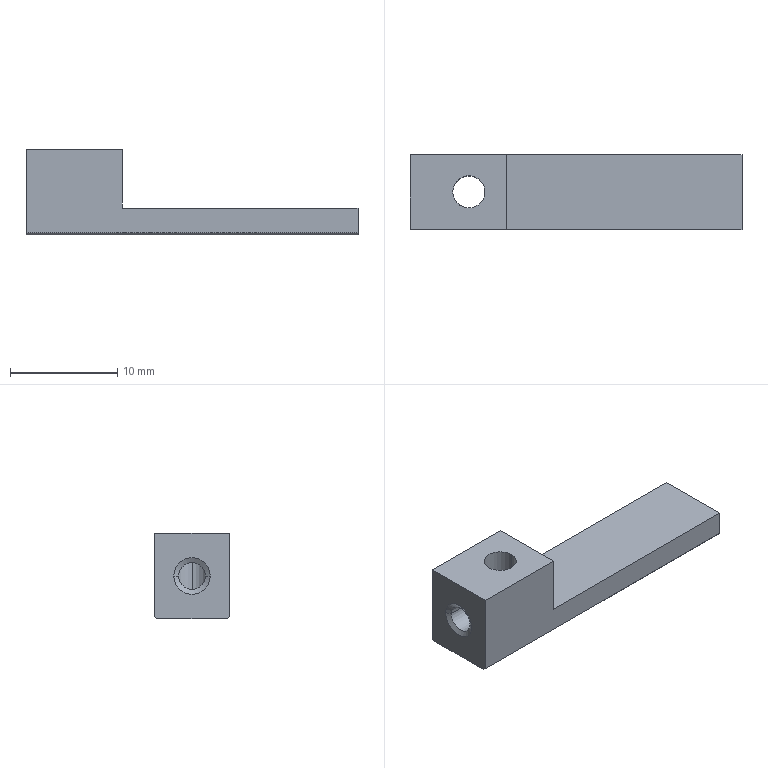Part | NX | 1 solid | 16 faces | box 31 x 7 x 8 mm | volume 810.336 mm3 | plane 10 | cylinder 4 | cone 2 | commonest cylinder face diameters 2.5 x2 3 x2
STEP:
#1=CARTESIAN_POINT('',(15.5,-3.3,-4.));
#2=VERTEX_POINT('',#1);
#3=CARTESIAN_POINT('',(-15.5,-3.3,-4.));
#4=VERTEX_POINT('',#3);
#5=CARTESIAN_POINT('',(0.,-3.3,-4.));
#6=DIRECTION('',(-1.,0.,0.));
#7=VECTOR('',#6,1000.);
#8=LINE('',#5,#7);
#9=EDGE_CURVE('',#2,#4,#8,.T.);
#10=ORIENTED_EDGE('',*,*,#9,.T.);
#11=CARTESIAN_POINT('',(-15.5,3.3,-4.));
#12=VERTEX_POINT('',#11);
#13=CARTESIAN_POINT('',(-15.5,0.,-4.));
#14=DIRECTION('',(0.,-1.,0.));
#15=VECTOR('',#14,1000.);
#16=LINE('',#13,#15);
#17=EDGE_CURVE('',#12,#4,#16,.T.);
#18=ORIENTED_EDGE('',*,*,#17,.F.);
#19=CARTESIAN_POINT('',(15.5,3.3,-4.));
#20=VERTEX_POINT('',#19);
#21=CARTESIAN_POINT('',(0.,3.3,-4.));
#22=DIRECTION('',(1.,0.,0.));
#23=VECTOR('',#22,1000.);
#24=LINE('',#21,#23);
#25=EDGE_CURVE('',#12,#20,#24,.T.);
#26=ORIENTED_EDGE('',*,*,#25,.T.);
#27=CARTESIAN_POINT('',(15.5,3.5,-4.));
#28=DIRECTION('',(0.,-1.,0.));
#29=VECTOR('',#28,1000.);
#30=LINE('',#27,#29);
#31=EDGE_CURVE('',#20,#2,#30,.T.);
#32=ORIENTED_EDGE('',*,*,#31,.T.);
#33=EDGE_LOOP('',(#10,#18,#26,#32));
#34=FACE_BOUND('',#33,.T.);
#35=CARTESIAN_POINT('',(-11.5,0.,-4.));
#36=VERTEX_POINT('',#35);
#37=CARTESIAN_POINT('',(-8.5,0.,-4.));
#38=VERTEX_POINT('',#37);
#39=CARTESIAN_POINT('',(-10.,0.,-4.));
#40=DIRECTION('',(0.,0.,1.));
#41=DIRECTION('',(1.,0.,0.));
#42=AXIS2_PLACEMENT_3D('',#39,#40,#41);
#43=CIRCLE('',#42,1.5);
#44=EDGE_CURVE('',#36,#38,#43,.T.);
#45=ORIENTED_EDGE('',*,*,#44,.T.);
#46=CARTESIAN_POINT('',(-10.,0.,-4.));
#47=DIRECTION('',(0.,0.,1.));
#48=DIRECTION('',(1.,0.,0.));
#49=AXIS2_PLACEMENT_3D('',#46,#47,#48);
#50=CIRCLE('',#49,1.5);
#51=EDGE_CURVE('',#38,#36,#50,.T.);
#52=ORIENTED_EDGE('',*,*,#51,.T.);
#53=EDGE_LOOP('',(#45,#52));
#54=FACE_BOUND('',#53,.T.);
#55=CARTESIAN_POINT('',(0.,0.,-4.));
#56=DIRECTION('',(0.,0.,1.));
#57=DIRECTION('',(1.,0.,0.));
#58=AXIS2_PLACEMENT_3D('',#55,#56,#57);
#59=PLANE('',#58);
#60=ADVANCED_FACE('',(#34,#54),#59,.F.);
#61=ORIENTED_EDGE('',*,*,#17,.T.);
#62=CARTESIAN_POINT('',(-15.5,-3.5,-3.8));
#63=VERTEX_POINT('',#62);
#64=CARTESIAN_POINT('',(-15.5,-7.3,0.));
#65=DIRECTION('',(0.,0.7071,-0.7071));
#66=VECTOR('',#65,1000.);
#67=LINE('',#64,#66);
#68=EDGE_CURVE('',#63,#4,#67,.T.);
#69=ORIENTED_EDGE('',*,*,#68,.F.);
#70=CARTESIAN_POINT('',(-15.5,-3.5,4.));
#71=VERTEX_POINT('',#70);
#72=CARTESIAN_POINT('',(-15.5,-3.5,0.));
#73=DIRECTION('',(0.,0.,-1.));
#74=VECTOR('',#73,1000.);
#75=LINE('',#72,#74);
#76=EDGE_CURVE('',#71,#63,#75,.T.);
#77=ORIENTED_EDGE('',*,*,#76,.F.);
#78=CARTESIAN_POINT('',(-15.5,3.5,4.));
#79=VERTEX_POINT('',#78);
#80=CARTESIAN_POINT('',(-15.5,0.,4.));
#81=DIRECTION('',(0.,-1.,0.));
#82=VECTOR('',#81,1000.);
#83=LINE('',#80,#82);
#84=EDGE_CURVE('',#79,#71,#83,.T.);
#85=ORIENTED_EDGE('',*,*,#84,.F.);
#86=CARTESIAN_POINT('',(-15.5,3.5,-3.8));
#87=VERTEX_POINT('',#86);
#88=CARTESIAN_POINT('',(-15.5,3.5,0.));
#89=DIRECTION('',(0.,0.,1.));
#90=VECTOR('',#89,1000.);
#91=LINE('',#88,#90);
#92=EDGE_CURVE('',#87,#79,#91,.T.);
#93=ORIENTED_EDGE('',*,*,#92,.F.);
#94=CARTESIAN_POINT('',(-15.5,7.3,0.));
#95=DIRECTION('',(0.,0.7071,0.7071));
#96=VECTOR('',#95,1000.);
#97=LINE('',#94,#96);
#98=EDGE_CURVE('',#12,#87,#97,.T.);
#99=ORIENTED_EDGE('',*,*,#98,.F.);
#100=EDGE_LOOP('',(#61,#69,#77,#85,#93,#99));
#101=FACE_BOUND('',#100,.T.);
#102=CARTESIAN_POINT('',(-15.5,1.7,0.));
#103=VERTEX_POINT('',#102);
#104=CARTESIAN_POINT('',(-15.5,-1.7,0.));
#105=VERTEX_POINT('',#104);
#106=CARTESIAN_POINT('',(-15.5,0.,0.));
#107=DIRECTION('',(-1.,0.,0.));
#108=DIRECTION('',(0.,1.,0.));
#109=AXIS2_PLACEMENT_3D('',#106,#107,#108);
#110=CIRCLE('',#109,1.7);
#111=EDGE_CURVE('',#103,#105,#110,.T.);
#112=ORIENTED_EDGE('',*,*,#111,.F.);
#113=CARTESIAN_POINT('',(-15.5,0.,0.));
#114=DIRECTION('',(-1.,0.,0.));
#115=DIRECTION('',(0.,1.,0.));
#116=AXIS2_PLACEMENT_3D('',#113,#114,#115);
#117=CIRCLE('',#116,1.7);
#118=EDGE_CURVE('',#105,#103,#117,.T.);
#119=ORIENTED_EDGE('',*,*,#118,.F.);
#120=EDGE_LOOP('',(#112,#119));
#121=FACE_BOUND('',#120,.T.);
#122=CARTESIAN_POINT('',(-15.5,3.5,-4.));
#123=DIRECTION('',(-1.,0.,0.));
#124=DIRECTION('',(0.,0.,1.));
#125=AXIS2_PLACEMENT_3D('',#122,#123,#124);
#126=PLANE('',#125);
#127=ADVANCED_FACE('',(#101,#121),#126,.T.);
#128=CARTESIAN_POINT('',(-6.5,3.5,-1.5));
#129=VERTEX_POINT('',#128);
#130=CARTESIAN_POINT('',(15.5,3.5,-1.5));
#131=VERTEX_POINT('',#130);
#132=CARTESIAN_POINT('',(-6.5,3.5,-1.5));
#133=DIRECTION('',(1.,0.,0.));
#134=VECTOR('',#133,1000.);
#135=LINE('',#132,#134);
#136=EDGE_CURVE('',#129,#131,#135,.T.);
#137=ORIENTED_EDGE('',*,*,#136,.T.);
#138=CARTESIAN_POINT('',(15.5,3.5,-3.8));
#139=VERTEX_POINT('',#138);
#140=CARTESIAN_POINT('',(15.5,3.5,-1.5));
#141=DIRECTION('',(0.,0.,-1.));
#142=VECTOR('',#141,1000.);
#143=LINE('',#140,#142);
#144=EDGE_CURVE('',#131,#139,#143,.T.);
#145=ORIENTED_EDGE('',*,*,#144,.T.);
#146=CARTESIAN_POINT('',(0.,3.5,-3.8));
#147=DIRECTION('',(1.,0.,0.));
#148=VECTOR('',#147,1000.);
#149=LINE('',#146,#148);
#150=EDGE_CURVE('',#87,#139,#149,.T.);
#151=ORIENTED_EDGE('',*,*,#150,.F.);
#152=ORIENTED_EDGE('',*,*,#92,.T.);
#153=CARTESIAN_POINT('',(-6.5,3.5,4.));
#154=VERTEX_POINT('',#153);
#155=CARTESIAN_POINT('',(-15.5,3.5,4.));
#156=DIRECTION('',(1.,0.,0.));
#157=VECTOR('',#156,1000.);
#158=LINE('',#155,#157);
#159=EDGE_CURVE('',#79,#154,#158,.T.);
#160=ORIENTED_EDGE('',*,*,#159,.T.);
#161=CARTESIAN_POINT('',(-6.5,3.5,-1.5));
#162=DIRECTION('',(0.,0.,1.));
#163=VECTOR('',#162,1000.);
#164=LINE('',#161,#163);
#165=EDGE_CURVE('',#129,#154,#164,.T.);
#166=ORIENTED_EDGE('',*,*,#165,.F.);
#167=EDGE_LOOP('',(#137,#145,#151,#152,#160,#166));
#168=FACE_BOUND('',#167,.T.);
#169=CARTESIAN_POINT('',(15.5,3.5,-4.));
#170=DIRECTION('',(0.,1.,0.));
#171=DIRECTION('',(1.,0.,0.));
#172=AXIS2_PLACEMENT_3D('',#169,#170,#171);
#173=PLANE('',#172);
#174=ADVANCED_FACE('',(#168),#173,.T.);
#175=CARTESIAN_POINT('',(-6.5,-3.5,-1.5));
#176=VERTEX_POINT('',#175);
#177=CARTESIAN_POINT('',(15.5,-3.5,-1.5));
#178=VERTEX_POINT('',#177);
#179=CARTESIAN_POINT('',(-6.5,-3.5,-1.5));
#180=DIRECTION('',(1.,0.,0.));
#181=VECTOR('',#180,1000.);
#182=LINE('',#179,#181);
#183=EDGE_CURVE('',#176,#178,#182,.T.);
#184=ORIENTED_EDGE('',*,*,#183,.T.);
#185=CARTESIAN_POINT('',(15.5,3.5,-1.5));
#186=DIRECTION('',(0.,-1.,0.));
#187=VECTOR('',#186,1000.);
#188=LINE('',#185,#187);
#189=EDGE_CURVE('',#131,#178,#188,.T.);
#190=ORIENTED_EDGE('',*,*,#189,.F.);
#191=ORIENTED_EDGE('',*,*,#136,.F.);
#192=CARTESIAN_POINT('',(-6.5,-3.5,-1.5));
#193=DIRECTION('',(0.,1.,0.));
#194=VECTOR('',#193,1000.);
#195=LINE('',#192,#194);
#196=EDGE_CURVE('',#176,#129,#195,.T.);
#197=ORIENTED_EDGE('',*,*,#196,.F.);
#198=EDGE_LOOP('',(#184,#190,#191,#197));
#199=FACE_BOUND('',#198,.T.);
#200=CARTESIAN_POINT('',(15.5,3.5,-1.5));
#201=DIRECTION('',(0.,0.,-1.));
#202=DIRECTION('',(0.,-1.,0.));
#203=AXIS2_PLACEMENT_3D('',#200,#201,#202);
#204=PLANE('',#203);
#205=ADVANCED_FACE('',(#199),#204,.F.);
#206=ORIENTED_EDGE('',*,*,#183,.F.);
#207=CARTESIAN_POINT('',(-6.5,-3.5,4.));
#208=VERTEX_POINT('',#207);
#209=CARTESIAN_POINT('',(-6.5,-3.5,-1.5));
#210=DIRECTION('',(0.,0.,1.));
#211=VECTOR('',#210,1000.);
#212=LINE('',#209,#211);
#213=EDGE_CURVE('',#176,#208,#212,.T.);
#214=ORIENTED_EDGE('',*,*,#213,.T.);
#215=CARTESIAN_POINT('',(-6.5,-3.5,4.));
#216=DIRECTION('',(-1.,0.,0.));
#217=VECTOR('',#216,1000.);
#218=LINE('',#215,#217);
#219=EDGE_CURVE('',#208,#71,#218,.T.);
#220=ORIENTED_EDGE('',*,*,#219,.T.);
#221=ORIENTED_EDGE('',*,*,#76,.T.);
#222=CARTESIAN_POINT('',(15.5,-3.5,-3.8));
#223=VERTEX_POINT('',#222);
#224=CARTESIAN_POINT('',(0.,-3.5,-3.8));
#225=DIRECTION('',(-1.,0.,0.));
#226=VECTOR('',#225,1000.);
#227=LINE('',#224,#226);
#228=EDGE_CURVE('',#223,#63,#227,.T.);
#229=ORIENTED_EDGE('',*,*,#228,.F.);
#230=CARTESIAN_POINT('',(15.5,-3.5,-1.5));
#231=DIRECTION('',(0.,0.,-1.));
#232=VECTOR('',#231,1000.);
#233=LINE('',#230,#232);
#234=EDGE_CURVE('',#178,#223,#233,.T.);
#235=ORIENTED_EDGE('',*,*,#234,.F.);
#236=EDGE_LOOP('',(#206,#214,#220,#221,#229,#235));
#237=FACE_BOUND('',#236,.T.);
#238=CARTESIAN_POINT('',(-15.5,-3.5,-4.));
#239=DIRECTION('',(0.,-1.,0.));
#240=DIRECTION('',(0.,0.,-1.));
#241=AXIS2_PLACEMENT_3D('',#238,#239,#240);
#242=PLANE('',#241);
#243=ADVANCED_FACE('',(#237),#242,.T.);
#244=ORIENTED_EDGE('',*,*,#189,.T.);
#245=ORIENTED_EDGE('',*,*,#234,.T.);
#246=CARTESIAN_POINT('',(15.5,-7.3,0.));
#247=DIRECTION('',(0.,-0.7071,0.7071));
#248=VECTOR('',#247,1000.);
#249=LINE('',#246,#248);
#250=EDGE_CURVE('',#2,#223,#249,.T.);
#251=ORIENTED_EDGE('',*,*,#250,.F.);
#252=ORIENTED_EDGE('',*,*,#31,.F.);
#253=CARTESIAN_POINT('',(15.5,7.3,0.));
#254=DIRECTION('',(0.,-0.7071,-0.7071));
#255=VECTOR('',#254,1000.);
#256=LINE('',#253,#255);
#257=EDGE_CURVE('',#139,#20,#256,.T.);
#258=ORIENTED_EDGE('',*,*,#257,.F.);
#259=ORIENTED_EDGE('',*,*,#144,.F.);
#260=EDGE_LOOP('',(#244,#245,#251,#252,#258,#259));
#261=FACE_BOUND('',#260,.T.);
#262=CARTESIAN_POINT('',(15.5,-3.5,-4.));
#263=DIRECTION('',(1.,0.,0.));
#264=DIRECTION('',(0.,1.,0.));
#265=AXIS2_PLACEMENT_3D('',#262,#263,#264);
#266=PLANE('',#265);
#267=ADVANCED_FACE('',(#261),#266,.T.);
#268=CARTESIAN_POINT('',(-6.5,3.5,4.));
#269=DIRECTION('',(0.,-1.,0.));
#270=VECTOR('',#269,1000.);
#271=LINE('',#268,#270);
#272=EDGE_CURVE('',#154,#208,#271,.T.);
#273=ORIENTED_EDGE('',*,*,#272,.F.);
#274=ORIENTED_EDGE('',*,*,#159,.F.);
#275=ORIENTED_EDGE('',*,*,#84,.T.);
#276=ORIENTED_EDGE('',*,*,#219,.F.);
#277=EDGE_LOOP('',(#273,#274,#275,#276));
#278=FACE_BOUND('',#277,.T.);
#279=CARTESIAN_POINT('',(-8.5,0.,4.));
#280=VERTEX_POINT('',#279);
#281=CARTESIAN_POINT('',(-11.5,0.,4.));
#282=VERTEX_POINT('',#281);
#283=CARTESIAN_POINT('',(-10.,0.,4.));
#284=DIRECTION('',(0.,0.,1.));
#285=DIRECTION('',(1.,0.,0.));
#286=AXIS2_PLACEMENT_3D('',#283,#284,#285);
#287=CIRCLE('',#286,1.5);
#288=EDGE_CURVE('',#280,#282,#287,.T.);
#289=ORIENTED_EDGE('',*,*,#288,.F.);
#290=CARTESIAN_POINT('',(-10.,0.,4.));
#291=DIRECTION('',(0.,0.,1.));
#292=DIRECTION('',(1.,0.,0.));
#293=AXIS2_PLACEMENT_3D('',#290,#291,#292);
#294=CIRCLE('',#293,1.5);
#295=EDGE_CURVE('',#282,#280,#294,.T.);
#296=ORIENTED_EDGE('',*,*,#295,.F.);
#297=EDGE_LOOP('',(#289,#296));
#298=FACE_BOUND('',#297,.T.);
#299=CARTESIAN_POINT('',(0.,0.,4.));
#300=DIRECTION('',(0.,0.,1.));
#301=DIRECTION('',(1.,0.,0.));
#302=AXIS2_PLACEMENT_3D('',#299,#300,#301);
#303=PLANE('',#302);
#304=ADVANCED_FACE('',(#278,#298),#303,.T.);
#305=ORIENTED_EDGE('',*,*,#272,.T.);
#306=ORIENTED_EDGE('',*,*,#213,.F.);
#307=ORIENTED_EDGE('',*,*,#196,.T.);
#308=ORIENTED_EDGE('',*,*,#165,.T.);
#309=EDGE_LOOP('',(#305,#306,#307,#308));
#310=FACE_BOUND('',#309,.T.);
#311=CARTESIAN_POINT('',(-6.5,3.5,-1.5));
#312=DIRECTION('',(-1.,0.,0.));
#313=DIRECTION('',(0.,0.,1.));
#314=AXIS2_PLACEMENT_3D('',#311,#312,#313);
#315=PLANE('',#314);
#316=ADVANCED_FACE('',(#310),#315,.F.);
#317=ORIENTED_EDGE('',*,*,#44,.F.);
#318=CARTESIAN_POINT('',(-11.5,0.,-1.25));
#319=VERTEX_POINT('',#318);
#320=CARTESIAN_POINT('',(-11.5,0.,-4.));
#321=DIRECTION('',(0.,0.,1.));
#322=VECTOR('',#321,1000.);
#323=LINE('',#320,#322);
#324=EDGE_CURVE('',#319,#36,#323,.F.);
#325=ORIENTED_EDGE('',*,*,#324,.F.);
#326=CARTESIAN_POINT('',(-10.829,-1.25,0.));
#327=VERTEX_POINT('',#326);
#328=CARTESIAN_POINT('',(-11.5,0.,-1.25));
#329=CARTESIAN_POINT('',(-11.5,-0.342,-1.25));
#330=CARTESIAN_POINT('',(-11.245,-0.9913,-0.9645));
#331=CARTESIAN_POINT('',(-10.83,-1.25,-0.3175));
#332=CARTESIAN_POINT('',(-10.829,-1.25,0.));
#333=B_SPLINE_CURVE_WITH_KNOTS('',3,(#328,#329,#330,#331,#332),.UNSPECIFIED.,.F.,.F.,(4,1,4),(0.,0.5,1.),.UNSPECIFIED.);
#334=EDGE_CURVE('',#319,#327,#333,.T.);
#335=ORIENTED_EDGE('',*,*,#334,.T.);
#336=CARTESIAN_POINT('',(-11.5,0.,1.25));
#337=VERTEX_POINT('',#336);
#338=CARTESIAN_POINT('',(-10.829,-1.25,0.));
#339=CARTESIAN_POINT('',(-10.83,-1.25,0.3174));
#340=CARTESIAN_POINT('',(-11.245,-0.9912,0.9645));
#341=CARTESIAN_POINT('',(-11.5,-0.3421,1.25));
#342=CARTESIAN_POINT('',(-11.5,0.,1.25));
#343=B_SPLINE_CURVE_WITH_KNOTS('',3,(#338,#339,#340,#341,#342),.UNSPECIFIED.,.F.,.F.,(4,1,4),(0.,0.5,1.),.UNSPECIFIED.);
#344=EDGE_CURVE('',#327,#337,#343,.T.);
#345=ORIENTED_EDGE('',*,*,#344,.T.);
#346=CARTESIAN_POINT('',(-11.5,0.,-4.));
#347=DIRECTION('',(0.,0.,1.));
#348=VECTOR('',#347,1000.);
#349=LINE('',#346,#348);
#350=EDGE_CURVE('',#337,#282,#349,.T.);
#351=ORIENTED_EDGE('',*,*,#350,.T.);
#352=ORIENTED_EDGE('',*,*,#295,.T.);
#353=CARTESIAN_POINT('',(-8.5,0.,-4.));
#354=DIRECTION('',(0.,0.,1.));
#355=VECTOR('',#354,1000.);
#356=LINE('',#353,#355);
#357=EDGE_CURVE('',#280,#38,#356,.F.);
#358=ORIENTED_EDGE('',*,*,#357,.T.);
#359=EDGE_LOOP('',(#317,#325,#335,#345,#351,#352,#358));
#360=FACE_BOUND('',#359,.T.);
#361=CARTESIAN_POINT('',(-10.,0.,-4.));
#362=DIRECTION('',(0.,0.,1.));
#363=DIRECTION('',(1.,0.,0.));
#364=AXIS2_PLACEMENT_3D('',#361,#362,#363);
#365=CYLINDRICAL_SURFACE('',#364,1.5);
#366=ADVANCED_FACE('',(#360),#365,.F.);
#367=ORIENTED_EDGE('',*,*,#344,.F.);
#368=CARTESIAN_POINT('',(-15.24,-1.25,0.));
#369=VERTEX_POINT('',#368);
#370=CARTESIAN_POINT('',(-15.5,-1.25,0.));
#371=DIRECTION('',(-1.,0.,0.));
#372=VECTOR('',#371,1000.);
#373=LINE('',#370,#372);
#374=EDGE_CURVE('',#327,#369,#373,.T.);
#375=ORIENTED_EDGE('',*,*,#374,.T.);
#376=CARTESIAN_POINT('',(-15.24,1.25,0.));
#377=VERTEX_POINT('',#376);
#378=CARTESIAN_POINT('',(-15.24,0.,0.));
#379=DIRECTION('',(-1.,0.,0.));
#380=DIRECTION('',(0.,1.,0.));
#381=AXIS2_PLACEMENT_3D('',#378,#379,#380);
#382=CIRCLE('',#381,1.25);
#383=EDGE_CURVE('',#369,#377,#382,.T.);
#384=ORIENTED_EDGE('',*,*,#383,.T.);
#385=CARTESIAN_POINT('',(-10.829,1.25,0.));
#386=VERTEX_POINT('',#385);
#387=CARTESIAN_POINT('',(-15.5,1.25,0.));
#388=DIRECTION('',(-1.,0.,0.));
#389=VECTOR('',#388,1000.);
#390=LINE('',#387,#389);
#391=EDGE_CURVE('',#386,#377,#390,.T.);
#392=ORIENTED_EDGE('',*,*,#391,.F.);
#393=CARTESIAN_POINT('',(-10.829,1.25,0.));
#394=CARTESIAN_POINT('',(-10.829,1.25,0.1449));
#395=CARTESIAN_POINT('',(-10.935,1.174,0.4572));
#396=CARTESIAN_POINT('',(-11.039,1.09,0.6325));
#397=CARTESIAN_POINT('',(-11.182,0.9256,0.8438));
#398=CARTESIAN_POINT('',(-11.202,0.8996,0.8699));
#399=CARTESIAN_POINT('',(-11.345,0.6794,1.063));
#400=CARTESIAN_POINT('',(-11.438,0.4603,1.174));
#401=CARTESIAN_POINT('',(-11.5,0.1667,1.25));
#402=CARTESIAN_POINT('',(-11.5,0.,1.25));
#403=B_SPLINE_CURVE_WITH_KNOTS('',3,(#393,#394,#395,#396,#397,#398,#399,#400,#401,#402),.UNSPECIFIED.,.F.,.F.,(4,1,1,1,1,1,1,4),(0.,0.25,0.375,0.4375,0.5,0.625,0.75,1.),.UNSPECIFIED.);
#404=EDGE_CURVE('',#337,#386,#403,.F.);
#405=ORIENTED_EDGE('',*,*,#404,.F.);
#406=EDGE_LOOP('',(#367,#375,#384,#392,#405));
#407=FACE_BOUND('',#406,.T.);
#408=CARTESIAN_POINT('',(-15.5,0.,0.));
#409=DIRECTION('',(-1.,0.,0.));
#410=DIRECTION('',(0.,1.,0.));
#411=AXIS2_PLACEMENT_3D('',#408,#409,#410);
#412=CYLINDRICAL_SURFACE('',#411,1.25);
#413=ADVANCED_FACE('',(#407),#412,.F.);
#414=ORIENTED_EDGE('',*,*,#111,.T.);
#415=CARTESIAN_POINT('',(-15.24,-1.25,0.));
#416=DIRECTION('',(-0.5,-0.866,0.));
#417=VECTOR('',#416,1000.);
#418=LINE('',#415,#417);
#419=EDGE_CURVE('',#105,#369,#418,.F.);
#420=ORIENTED_EDGE('',*,*,#419,.T.);
#421=CARTESIAN_POINT('',(-15.24,0.,0.));
#422=DIRECTION('',(-1.,0.,0.));
#423=DIRECTION('',(0.,1.,0.));
#424=AXIS2_PLACEMENT_3D('',#421,#422,#423);
#425=CIRCLE('',#424,1.25);
#426=EDGE_CURVE('',#377,#369,#425,.T.);
#427=ORIENTED_EDGE('',*,*,#426,.F.);
#428=CARTESIAN_POINT('',(-15.24,1.25,0.));
#429=DIRECTION('',(-0.5,0.866,0.));
#430=VECTOR('',#429,1000.);
#431=LINE('',#428,#430);
#432=EDGE_CURVE('',#103,#377,#431,.F.);
#433=ORIENTED_EDGE('',*,*,#432,.F.);
#434=EDGE_LOOP('',(#414,#420,#427,#433));
#435=FACE_BOUND('',#434,.T.);
#436=CARTESIAN_POINT('',(-15.24,0.,0.));
#437=DIRECTION('',(-1.,0.,0.));
#438=DIRECTION('',(0.,1.,0.));
#439=AXIS2_PLACEMENT_3D('',#436,#437,#438);
#440=CONICAL_SURFACE('',#439,1.25,1.047);
#441=ADVANCED_FACE('',(#435),#440,.F.);
#442=ORIENTED_EDGE('',*,*,#25,.F.);
#443=ORIENTED_EDGE('',*,*,#98,.T.);
#444=ORIENTED_EDGE('',*,*,#150,.T.);
#445=ORIENTED_EDGE('',*,*,#257,.T.);
#446=EDGE_LOOP('',(#442,#443,#444,#445));
#447=FACE_BOUND('',#446,.T.);
#448=CARTESIAN_POINT('',(0.,3.4,-3.9));
#449=DIRECTION('',(0.,0.7071,-0.7071));
#450=DIRECTION('',(-1.,0.,0.));
#451=AXIS2_PLACEMENT_3D('',#448,#449,#450);
#452=PLANE('',#451);
#453=ADVANCED_FACE('',(#447),#452,.T.);
#454=ORIENTED_EDGE('',*,*,#9,.F.);
#455=ORIENTED_EDGE('',*,*,#250,.T.);
#456=ORIENTED_EDGE('',*,*,#228,.T.);
#457=ORIENTED_EDGE('',*,*,#68,.T.);
#458=EDGE_LOOP('',(#454,#455,#456,#457));
#459=FACE_BOUND('',#458,.T.);
#460=CARTESIAN_POINT('',(0.,-3.4,-3.9));
#461=DIRECTION('',(0.,-0.7071,-0.7071));
#462=DIRECTION('',(0.,-0.7071,0.7071));
#463=AXIS2_PLACEMENT_3D('',#460,#461,#462);
#464=PLANE('',#463);
#465=ADVANCED_FACE('',(#459),#464,.T.);
#466=ORIENTED_EDGE('',*,*,#383,.F.);
#467=ORIENTED_EDGE('',*,*,#419,.F.);
#468=ORIENTED_EDGE('',*,*,#118,.T.);
#469=ORIENTED_EDGE('',*,*,#432,.T.);
#470=EDGE_LOOP('',(#466,#467,#468,#469));
#471=FACE_BOUND('',#470,.T.);
#472=CARTESIAN_POINT('',(-15.24,0.,0.));
#473=DIRECTION('',(-1.,0.,0.));
#474=DIRECTION('',(0.,1.,0.));
#475=AXIS2_PLACEMENT_3D('',#472,#473,#474);
#476=CONICAL_SURFACE('',#475,1.25,1.047);
#477=ADVANCED_FACE('',(#471),#476,.F.);
#478=ORIENTED_EDGE('',*,*,#391,.T.);
#479=ORIENTED_EDGE('',*,*,#426,.T.);
#480=ORIENTED_EDGE('',*,*,#374,.F.);
#481=ORIENTED_EDGE('',*,*,#334,.F.);
#482=CARTESIAN_POINT('',(-11.5,0.,-1.25));
#483=CARTESIAN_POINT('',(-11.5,0.1667,-1.25));
#484=CARTESIAN_POINT('',(-11.438,0.4604,-1.174));
#485=CARTESIAN_POINT('',(-11.345,0.6792,-1.063));
#486=CARTESIAN_POINT('',(-11.202,0.8998,-0.8698));
#487=CARTESIAN_POINT('',(-11.182,0.9253,-0.8441));
#488=CARTESIAN_POINT('',(-11.039,1.09,-0.6325));
#489=CARTESIAN_POINT('',(-10.935,1.173,-0.4548));
#490=CARTESIAN_POINT('',(-10.829,1.25,-0.1559));
#491=CARTESIAN_POINT('',(-10.829,1.25,0.));
#492=B_SPLINE_CURVE_WITH_KNOTS('',3,(#482,#483,#484,#485,#486,#487,#488,#489,#490,#491),.UNSPECIFIED.,.F.,.F.,(4,1,1,1,1,1,1,4),(0.,0.25,0.375,0.5,0.5625,0.625,0.75,1.),.UNSPECIFIED.);
#493=EDGE_CURVE('',#386,#319,#492,.F.);
#494=ORIENTED_EDGE('',*,*,#493,.F.);
#495=EDGE_LOOP('',(#478,#479,#480,#481,#494));
#496=FACE_BOUND('',#495,.T.);
#497=CARTESIAN_POINT('',(-15.5,0.,0.));
#498=DIRECTION('',(-1.,0.,0.));
#499=DIRECTION('',(0.,1.,0.));
#500=AXIS2_PLACEMENT_3D('',#497,#498,#499);
#501=CYLINDRICAL_SURFACE('',#500,1.25);
#502=ADVANCED_FACE('',(#496),#501,.F.);
#503=ORIENTED_EDGE('',*,*,#288,.T.);
#504=ORIENTED_EDGE('',*,*,#350,.F.);
#505=ORIENTED_EDGE('',*,*,#404,.T.);
#506=ORIENTED_EDGE('',*,*,#493,.T.);
#507=ORIENTED_EDGE('',*,*,#324,.T.);
#508=ORIENTED_EDGE('',*,*,#51,.F.);
#509=ORIENTED_EDGE('',*,*,#357,.F.);
#510=EDGE_LOOP('',(#503,#504,#505,#506,#507,#508,#509));
#511=FACE_BOUND('',#510,.T.);
#512=CARTESIAN_POINT('',(-10.,0.,-4.));
#513=DIRECTION('',(0.,0.,1.));
#514=DIRECTION('',(1.,0.,0.));
#515=AXIS2_PLACEMENT_3D('',#512,#513,#514);
#516=CYLINDRICAL_SURFACE('',#515,1.5);
#517=ADVANCED_FACE('',(#511),#516,.F.);
#518=CLOSED_SHELL('',(#60,#127,#174,#205,#243,#267,#304,#316,#366,#413,#441,#453,#465,#477,#502,#517));
#519=MANIFOLD_SOLID_BREP('',#518);
#520=(LENGTH_UNIT()NAMED_UNIT(*)SI_UNIT(.MILLI.,.METRE.));
#521=UNCERTAINTY_MEASURE_WITH_UNIT(LENGTH_MEASURE(0.0508),#520,'','');
#522=(NAMED_UNIT(*)PLANE_ANGLE_UNIT()SI_UNIT($,.RADIAN.));
#523=(NAMED_UNIT(*)SI_UNIT($,.STERADIAN.)SOLID_ANGLE_UNIT());
#524=(GEOMETRIC_REPRESENTATION_CONTEXT(3)GLOBAL_UNCERTAINTY_ASSIGNED_CONTEXT((#521))GLOBAL_UNIT_ASSIGNED_CONTEXT((#520,#522,#523))REPRESENTATION_CONTEXT('',''));
#525=ADVANCED_BREP_SHAPE_REPRESENTATION('',(#519),#524);